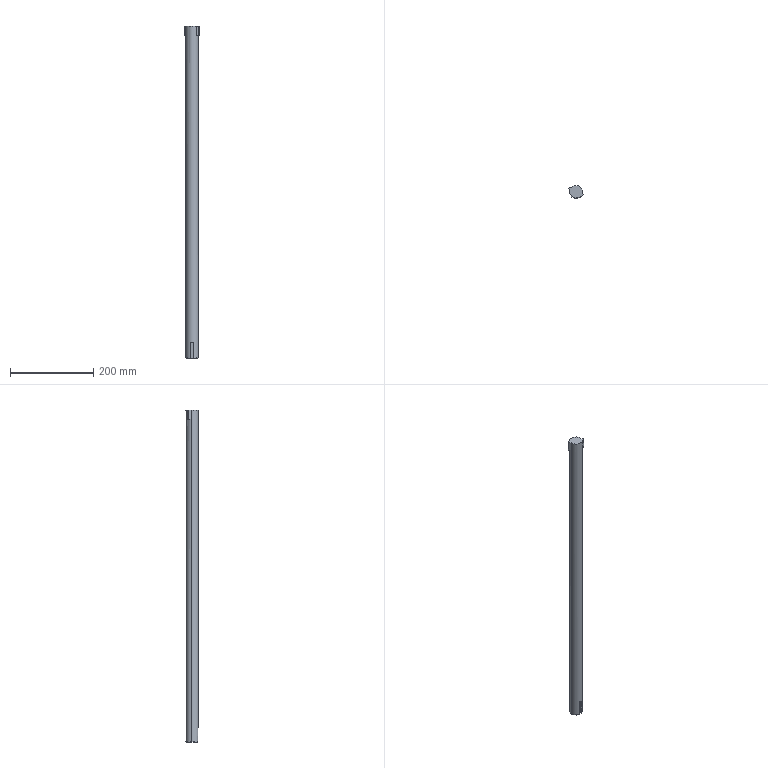Part | STEP file | SHAFT_DIA30_CARDANV11 | 1 solid | 20 faces | box 36.032 x 30 x 800 mm | volume 565605 mm3 | plane 13 | cylinder 4 | cone 3 | commonest cylinder face diameters 8 x2 30 x2